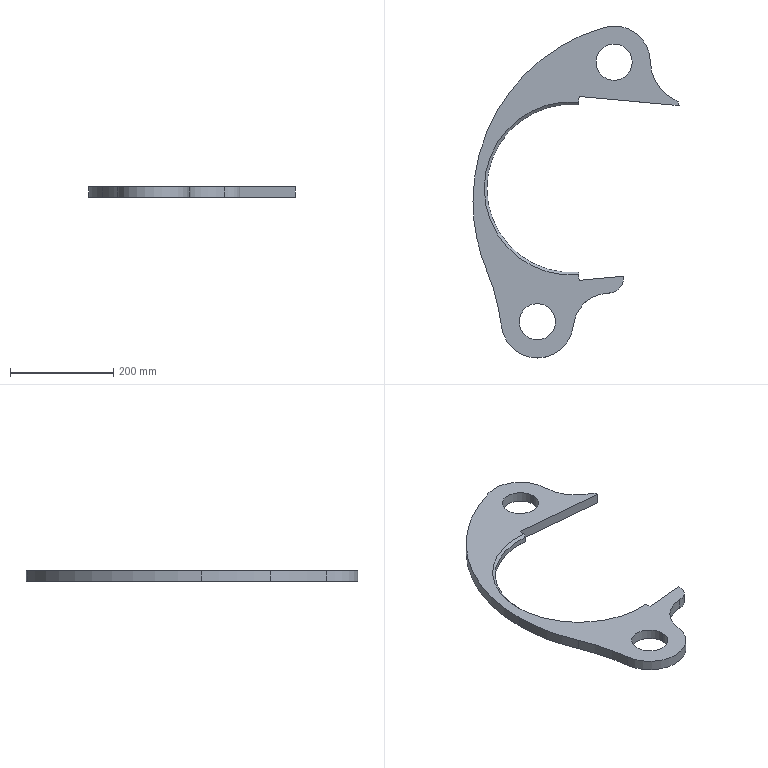Part | SolidWorks | features Chamfer 1, Extrusion 1 | 1 solid | 24 faces | box 398.626 x 642.2 x 20 mm | volume 1286836 mm3 | cylinder 15 | plane 6 | cone 3 | commonest cylinder face diameters 70 x4 140 x3 325 x2 700 x2 20 x1 60 x1
STEP:
#1=CARTESIAN_POINT('',(-162.5,0.,5.));
#2=VERTEX_POINT('',#1);
#3=CARTESIAN_POINT('',(14.745,161.83,5.));
#4=VERTEX_POINT('',#3);
#5=CARTESIAN_POINT('',(0.,0.,5.));
#6=DIRECTION('',(0.,0.,-1.));
#7=DIRECTION('',(1.,0.,0.));
#8=AXIS2_PLACEMENT_3D('',#5,#6,#7);
#9=CIRCLE('',#8,162.5);
#10=EDGE_CURVE('',#2,#4,#9,.T.);
#11=ORIENTED_EDGE('',*,*,#10,.F.);
#12=CARTESIAN_POINT('',(-167.5,0.,0.));
#13=VERTEX_POINT('',#12);
#14=CARTESIAN_POINT('',(-167.5,0.,0.));
#15=DIRECTION('',(-0.7071,0.,-0.7071));
#16=VECTOR('',#15,1000.);
#17=LINE('',#14,#16);
#18=EDGE_CURVE('',#2,#13,#17,.T.);
#19=ORIENTED_EDGE('',*,*,#18,.T.);
#20=CARTESIAN_POINT('',(15.199,166.809,0.));
#21=VERTEX_POINT('',#20);
#22=CARTESIAN_POINT('',(0.,0.,0.));
#23=DIRECTION('',(0.,0.,1.));
#24=DIRECTION('',(1.,0.,0.));
#25=AXIS2_PLACEMENT_3D('',#22,#23,#24);
#26=CIRCLE('',#25,167.5);
#27=EDGE_CURVE('',#21,#13,#26,.T.);
#28=ORIENTED_EDGE('',*,*,#27,.F.);
#29=CARTESIAN_POINT('',(0.,0.,167.5));
#30=DIRECTION('',(0.06416,0.7042,-0.7071));
#31=VECTOR('',#30,1000.);
#32=LINE('',#29,#31);
#33=EDGE_CURVE('',#4,#21,#32,.T.);
#34=ORIENTED_EDGE('',*,*,#33,.F.);
#35=EDGE_LOOP('',(#11,#19,#28,#34));
#36=FACE_OUTER_BOUND('',#35,.T.);
#37=CARTESIAN_POINT('',(0.,0.,0.));
#38=DIRECTION('',(0.,0.,-1.));
#39=DIRECTION('',(-1.,0.,0.));
#40=AXIS2_PLACEMENT_3D('',#37,#38,#39);
#41=CONICAL_SURFACE('',#40,167.5,0.7854);
#42=ADVANCED_FACE('',(#36),#41,.F.);
#43=CARTESIAN_POINT('',(48.7,244.2,20.));
#44=VERTEX_POINT('',#43);
#45=CARTESIAN_POINT('',(118.7,244.2,20.));
#46=VERTEX_POINT('',#45);
#47=CARTESIAN_POINT('',(83.7,244.2,20.));
#48=DIRECTION('',(0.,0.,1.));
#49=DIRECTION('',(1.,0.,0.));
#50=AXIS2_PLACEMENT_3D('',#47,#48,#49);
#51=CIRCLE('',#50,35.);
#52=EDGE_CURVE('',#44,#46,#51,.T.);
#53=ORIENTED_EDGE('',*,*,#52,.T.);
#54=CARTESIAN_POINT('',(118.7,244.2,0.));
#55=VERTEX_POINT('',#54);
#56=CARTESIAN_POINT('',(118.7,244.2,20.));
#57=DIRECTION('',(0.,0.,-1.));
#58=VECTOR('',#57,1000.);
#59=LINE('',#56,#58);
#60=EDGE_CURVE('',#46,#55,#59,.T.);
#61=ORIENTED_EDGE('',*,*,#60,.T.);
#62=CARTESIAN_POINT('',(48.7,244.2,0.));
#63=VERTEX_POINT('',#62);
#64=CARTESIAN_POINT('',(83.7,244.2,0.));
#65=DIRECTION('',(0.,0.,1.));
#66=DIRECTION('',(1.,0.,0.));
#67=AXIS2_PLACEMENT_3D('',#64,#65,#66);
#68=CIRCLE('',#67,35.);
#69=EDGE_CURVE('',#63,#55,#68,.T.);
#70=ORIENTED_EDGE('',*,*,#69,.F.);
#71=CARTESIAN_POINT('',(48.7,244.2,20.));
#72=DIRECTION('',(0.,0.,-1.));
#73=VECTOR('',#72,1000.);
#74=LINE('',#71,#73);
#75=EDGE_CURVE('',#44,#63,#74,.T.);
#76=ORIENTED_EDGE('',*,*,#75,.F.);
#77=EDGE_LOOP('',(#53,#61,#70,#76));
#78=FACE_OUTER_BOUND('',#77,.T.);
#79=CARTESIAN_POINT('',(83.7,244.2,20.));
#80=DIRECTION('',(0.,0.,-1.));
#81=DIRECTION('',(-1.,0.,0.));
#82=AXIS2_PLACEMENT_3D('',#79,#80,#81);
#83=CYLINDRICAL_SURFACE('',#82,35.);
#84=ADVANCED_FACE('',(#78),#83,.F.);
#85=CARTESIAN_POINT('',(-99.8,-258.,20.));
#86=VERTEX_POINT('',#85);
#87=CARTESIAN_POINT('',(-29.8,-258.,20.));
#88=VERTEX_POINT('',#87);
#89=CARTESIAN_POINT('',(-64.8,-258.,20.));
#90=DIRECTION('',(0.,0.,1.));
#91=DIRECTION('',(1.,0.,0.));
#92=AXIS2_PLACEMENT_3D('',#89,#90,#91);
#93=CIRCLE('',#92,35.);
#94=EDGE_CURVE('',#86,#88,#93,.T.);
#95=ORIENTED_EDGE('',*,*,#94,.T.);
#96=CARTESIAN_POINT('',(-29.8,-258.,0.));
#97=VERTEX_POINT('',#96);
#98=CARTESIAN_POINT('',(-29.8,-258.,20.));
#99=DIRECTION('',(0.,0.,-1.));
#100=VECTOR('',#99,1000.);
#101=LINE('',#98,#100);
#102=EDGE_CURVE('',#88,#97,#101,.T.);
#103=ORIENTED_EDGE('',*,*,#102,.T.);
#104=CARTESIAN_POINT('',(-99.8,-258.,0.));
#105=VERTEX_POINT('',#104);
#106=CARTESIAN_POINT('',(-64.8,-258.,0.));
#107=DIRECTION('',(0.,0.,1.));
#108=DIRECTION('',(1.,0.,0.));
#109=AXIS2_PLACEMENT_3D('',#106,#107,#108);
#110=CIRCLE('',#109,35.);
#111=EDGE_CURVE('',#105,#97,#110,.T.);
#112=ORIENTED_EDGE('',*,*,#111,.F.);
#113=CARTESIAN_POINT('',(-99.8,-258.,20.));
#114=DIRECTION('',(0.,0.,-1.));
#115=VECTOR('',#114,1000.);
#116=LINE('',#113,#115);
#117=EDGE_CURVE('',#86,#105,#116,.T.);
#118=ORIENTED_EDGE('',*,*,#117,.F.);
#119=EDGE_LOOP('',(#95,#103,#112,#118));
#120=FACE_OUTER_BOUND('',#119,.T.);
#121=CARTESIAN_POINT('',(-64.8,-258.,20.));
#122=DIRECTION('',(0.,0.,-1.));
#123=DIRECTION('',(-1.,0.,0.));
#124=AXIS2_PLACEMENT_3D('',#121,#122,#123);
#125=CYLINDRICAL_SURFACE('',#124,35.);
#126=ADVANCED_FACE('',(#120),#125,.F.);
#127=CARTESIAN_POINT('',(-189.285,-25.,20.));
#128=VERTEX_POINT('',#127);
#129=CARTESIAN_POINT('',(-162.312,-159.735,20.));
#130=VERTEX_POINT('',#129);
#131=CARTESIAN_POINT('',(160.715,-25.,20.));
#132=DIRECTION('',(0.,0.,1.));
#133=DIRECTION('',(1.,0.,0.));
#134=AXIS2_PLACEMENT_3D('',#131,#132,#133);
#135=CIRCLE('',#134,350.);
#136=EDGE_CURVE('',#128,#130,#135,.T.);
#137=ORIENTED_EDGE('',*,*,#136,.F.);
#138=CARTESIAN_POINT('',(-189.285,-25.,0.));
#139=VERTEX_POINT('',#138);
#140=CARTESIAN_POINT('',(-189.285,-25.,20.));
#141=DIRECTION('',(0.,0.,-1.));
#142=VECTOR('',#141,1000.);
#143=LINE('',#140,#142);
#144=EDGE_CURVE('',#128,#139,#143,.T.);
#145=ORIENTED_EDGE('',*,*,#144,.T.);
#146=CARTESIAN_POINT('',(-162.312,-159.735,0.));
#147=VERTEX_POINT('',#146);
#148=CARTESIAN_POINT('',(160.715,-25.,0.));
#149=DIRECTION('',(0.,0.,1.));
#150=DIRECTION('',(1.,0.,0.));
#151=AXIS2_PLACEMENT_3D('',#148,#149,#150);
#152=CIRCLE('',#151,350.);
#153=EDGE_CURVE('',#139,#147,#152,.T.);
#154=ORIENTED_EDGE('',*,*,#153,.T.);
#155=CARTESIAN_POINT('',(-162.312,-159.735,20.));
#156=DIRECTION('',(0.,0.,-1.));
#157=VECTOR('',#156,1000.);
#158=LINE('',#155,#157);
#159=EDGE_CURVE('',#130,#147,#158,.T.);
#160=ORIENTED_EDGE('',*,*,#159,.F.);
#161=EDGE_LOOP('',(#137,#145,#154,#160));
#162=FACE_OUTER_BOUND('',#161,.T.);
#163=CARTESIAN_POINT('',(160.715,-25.,20.));
#164=DIRECTION('',(0.,0.,-1.));
#165=DIRECTION('',(-1.,0.,0.));
#166=AXIS2_PLACEMENT_3D('',#163,#164,#165);
#167=CYLINDRICAL_SURFACE('',#166,350.);
#168=ADVANCED_FACE('',(#162),#167,.T.);
#169=CARTESIAN_POINT('',(14.745,161.83,15.));
#170=VERTEX_POINT('',#169);
#171=CARTESIAN_POINT('',(-162.5,0.,15.));
#172=VERTEX_POINT('',#171);
#173=CARTESIAN_POINT('',(0.,0.,15.));
#174=DIRECTION('',(0.,0.,1.));
#175=DIRECTION('',(1.,0.,0.));
#176=AXIS2_PLACEMENT_3D('',#173,#174,#175);
#177=CIRCLE('',#176,162.5);
#178=EDGE_CURVE('',#170,#172,#177,.T.);
#179=ORIENTED_EDGE('',*,*,#178,.T.);
#180=CARTESIAN_POINT('',(-162.5,0.,20.));
#181=DIRECTION('',(0.,0.,-1.));
#182=VECTOR('',#181,1000.);
#183=LINE('',#180,#182);
#184=EDGE_CURVE('',#172,#2,#183,.T.);
#185=ORIENTED_EDGE('',*,*,#184,.T.);
#186=ORIENTED_EDGE('',*,*,#10,.T.);
#187=CARTESIAN_POINT('',(14.745,161.83,20.));
#188=DIRECTION('',(0.,0.,-1.));
#189=VECTOR('',#188,1000.);
#190=LINE('',#187,#189);
#191=EDGE_CURVE('',#170,#4,#190,.T.);
#192=ORIENTED_EDGE('',*,*,#191,.F.);
#193=EDGE_LOOP('',(#179,#185,#186,#192));
#194=FACE_OUTER_BOUND('',#193,.T.);
#195=CARTESIAN_POINT('',(0.,0.,20.));
#196=DIRECTION('',(0.,0.,-1.));
#197=DIRECTION('',(-1.,0.,0.));
#198=AXIS2_PLACEMENT_3D('',#195,#196,#197);
#199=CYLINDRICAL_SURFACE('',#198,162.5);
#200=ADVANCED_FACE('',(#194),#199,.F.);
#201=CARTESIAN_POINT('',(72.887,-202.606,0.));
#202=VERTEX_POINT('',#201);
#203=CARTESIAN_POINT('',(4.819,-265.294,0.));
#204=VERTEX_POINT('',#203);
#205=CARTESIAN_POINT('',(74.438,-272.588,0.));
#206=DIRECTION('',(0.,0.,1.));
#207=DIRECTION('',(1.,0.,0.));
#208=AXIS2_PLACEMENT_3D('',#205,#206,#207);
#209=CIRCLE('',#208,70.);
#210=EDGE_CURVE('',#202,#204,#209,.T.);
#211=ORIENTED_EDGE('',*,*,#210,.F.);
#212=CARTESIAN_POINT('',(72.887,-202.606,20.));
#213=VERTEX_POINT('',#212);
#214=CARTESIAN_POINT('',(72.887,-202.606,20.));
#215=DIRECTION('',(0.,0.,-1.));
#216=VECTOR('',#215,1000.);
#217=LINE('',#214,#216);
#218=EDGE_CURVE('',#213,#202,#217,.T.);
#219=ORIENTED_EDGE('',*,*,#218,.F.);
#220=CARTESIAN_POINT('',(4.819,-265.294,20.));
#221=VERTEX_POINT('',#220);
#222=CARTESIAN_POINT('',(74.438,-272.588,20.));
#223=DIRECTION('',(0.,0.,1.));
#224=DIRECTION('',(1.,0.,0.));
#225=AXIS2_PLACEMENT_3D('',#222,#223,#224);
#226=CIRCLE('',#225,70.);
#227=EDGE_CURVE('',#213,#221,#226,.T.);
#228=ORIENTED_EDGE('',*,*,#227,.T.);
#229=CARTESIAN_POINT('',(4.819,-265.294,20.));
#230=DIRECTION('',(0.,0.,-1.));
#231=VECTOR('',#230,1000.);
#232=LINE('',#229,#231);
#233=EDGE_CURVE('',#221,#204,#232,.T.);
#234=ORIENTED_EDGE('',*,*,#233,.T.);
#235=EDGE_LOOP('',(#211,#219,#228,#234));
#236=FACE_OUTER_BOUND('',#235,.T.);
#237=CARTESIAN_POINT('',(74.438,-272.588,20.));
#238=DIRECTION('',(0.,0.,-1.));
#239=DIRECTION('',(-1.,0.,0.));
#240=AXIS2_PLACEMENT_3D('',#237,#238,#239);
#241=CYLINDRICAL_SURFACE('',#240,70.);
#242=ADVANCED_FACE('',(#236),#241,.F.);
#243=CARTESIAN_POINT('',(102.1,-169.9,0.));
#244=VERTEX_POINT('',#243);
#245=CARTESIAN_POINT('',(72.223,-172.613,0.));
#246=DIRECTION('',(0.,0.,1.));
#247=DIRECTION('',(1.,0.,0.));
#248=AXIS2_PLACEMENT_3D('',#245,#246,#247);
#249=CIRCLE('',#248,30.);
#250=EDGE_CURVE('',#202,#244,#249,.T.);
#251=ORIENTED_EDGE('',*,*,#250,.T.);
#252=CARTESIAN_POINT('',(102.1,-169.9,20.));
#253=VERTEX_POINT('',#252);
#254=CARTESIAN_POINT('',(102.1,-169.9,20.));
#255=DIRECTION('',(0.,0.,-1.));
#256=VECTOR('',#255,1000.);
#257=LINE('',#254,#256);
#258=EDGE_CURVE('',#253,#244,#257,.T.);
#259=ORIENTED_EDGE('',*,*,#258,.F.);
#260=CARTESIAN_POINT('',(72.223,-172.613,20.));
#261=DIRECTION('',(0.,0.,1.));
#262=DIRECTION('',(1.,0.,0.));
#263=AXIS2_PLACEMENT_3D('',#260,#261,#262);
#264=CIRCLE('',#263,30.);
#265=EDGE_CURVE('',#213,#253,#264,.T.);
#266=ORIENTED_EDGE('',*,*,#265,.F.);
#267=ORIENTED_EDGE('',*,*,#218,.T.);
#268=EDGE_LOOP('',(#251,#259,#266,#267));
#269=FACE_OUTER_BOUND('',#268,.T.);
#270=CARTESIAN_POINT('',(72.223,-172.613,20.));
#271=DIRECTION('',(0.,0.,-1.));
#272=DIRECTION('',(-1.,0.,0.));
#273=AXIS2_PLACEMENT_3D('',#270,#271,#272);
#274=CYLINDRICAL_SURFACE('',#273,30.);
#275=ADVANCED_FACE('',(#269),#274,.T.);
#276=CARTESIAN_POINT('',(16.2,-177.7,0.));
#277=VERTEX_POINT('',#276);
#278=CARTESIAN_POINT('',(-28.351,-181.745,0.));
#279=DIRECTION('',(0.9959,0.09043,0.));
#280=VECTOR('',#279,1000.);
#281=LINE('',#278,#280);
#282=EDGE_CURVE('',#277,#244,#281,.T.);
#283=ORIENTED_EDGE('',*,*,#282,.F.);
#284=CARTESIAN_POINT('',(16.2,-177.7,20.));
#285=VERTEX_POINT('',#284);
#286=CARTESIAN_POINT('',(16.2,-177.7,20.));
#287=DIRECTION('',(0.,0.,-1.));
#288=VECTOR('',#287,1000.);
#289=LINE('',#286,#288);
#290=EDGE_CURVE('',#285,#277,#289,.T.);
#291=ORIENTED_EDGE('',*,*,#290,.F.);
#292=CARTESIAN_POINT('',(-28.351,-181.745,20.));
#293=DIRECTION('',(0.9959,0.09043,0.));
#294=VECTOR('',#293,1000.);
#295=LINE('',#292,#294);
#296=EDGE_CURVE('',#285,#253,#295,.T.);
#297=ORIENTED_EDGE('',*,*,#296,.T.);
#298=ORIENTED_EDGE('',*,*,#258,.T.);
#299=EDGE_LOOP('',(#283,#291,#297,#298));
#300=FACE_OUTER_BOUND('',#299,.T.);
#301=CARTESIAN_POINT('',(-28.351,-181.745,20.));
#302=DIRECTION('',(-0.09043,0.9959,0.));
#303=DIRECTION('',(-0.9959,-0.09043,0.));
#304=AXIS2_PLACEMENT_3D('',#301,#302,#303);
#305=PLANE('',#304);
#306=ADVANCED_FACE('',(#300),#305,.T.);
#307=CARTESIAN_POINT('',(15.207,-166.808,0.));
#308=VERTEX_POINT('',#307);
#309=CARTESIAN_POINT('',(54.115,-593.599,0.));
#310=DIRECTION('',(-0.09079,0.9959,0.));
#311=VECTOR('',#310,1000.);
#312=LINE('',#309,#311);
#313=EDGE_CURVE('',#277,#308,#312,.T.);
#314=ORIENTED_EDGE('',*,*,#313,.T.);
#315=CARTESIAN_POINT('',(14.753,-161.829,5.));
#316=VERTEX_POINT('',#315);
#317=CARTESIAN_POINT('',(0.,0.,167.5));
#318=DIRECTION('',(-0.0642,0.7042,0.7071));
#319=VECTOR('',#318,1000.);
#320=LINE('',#317,#319);
#321=EDGE_CURVE('',#308,#316,#320,.T.);
#322=ORIENTED_EDGE('',*,*,#321,.T.);
#323=CARTESIAN_POINT('',(14.753,-161.829,15.));
#324=VERTEX_POINT('',#323);
#325=CARTESIAN_POINT('',(14.753,-161.829,20.));
#326=DIRECTION('',(0.,0.,-1.));
#327=VECTOR('',#326,1000.);
#328=LINE('',#325,#327);
#329=EDGE_CURVE('',#324,#316,#328,.T.);
#330=ORIENTED_EDGE('',*,*,#329,.F.);
#331=CARTESIAN_POINT('',(15.207,-166.808,20.));
#332=VERTEX_POINT('',#331);
#333=CARTESIAN_POINT('',(0.,0.,-147.5));
#334=DIRECTION('',(0.0642,-0.7042,0.7071));
#335=VECTOR('',#334,1000.);
#336=LINE('',#333,#335);
#337=EDGE_CURVE('',#324,#332,#336,.T.);
#338=ORIENTED_EDGE('',*,*,#337,.T.);
#339=CARTESIAN_POINT('',(54.115,-593.599,20.));
#340=DIRECTION('',(-0.09079,0.9959,0.));
#341=VECTOR('',#340,1000.);
#342=LINE('',#339,#341);
#343=EDGE_CURVE('',#285,#332,#342,.T.);
#344=ORIENTED_EDGE('',*,*,#343,.F.);
#345=ORIENTED_EDGE('',*,*,#290,.T.);
#346=EDGE_LOOP('',(#314,#322,#330,#338,#344,#345));
#347=FACE_OUTER_BOUND('',#346,.T.);
#348=CARTESIAN_POINT('',(54.115,-593.599,20.));
#349=DIRECTION('',(-0.9959,-0.09079,0.));
#350=DIRECTION('',(0.09079,-0.9959,0.));
#351=AXIS2_PLACEMENT_3D('',#348,#349,#350);
#352=PLANE('',#351);
#353=ADVANCED_FACE('',(#347),#352,.F.);
#354=ORIENTED_EDGE('',*,*,#184,.F.);
#355=CARTESIAN_POINT('',(0.,0.,15.));
#356=DIRECTION('',(0.,0.,1.));
#357=DIRECTION('',(1.,0.,0.));
#358=AXIS2_PLACEMENT_3D('',#355,#356,#357);
#359=CIRCLE('',#358,162.5);
#360=EDGE_CURVE('',#172,#324,#359,.T.);
#361=ORIENTED_EDGE('',*,*,#360,.T.);
#362=ORIENTED_EDGE('',*,*,#329,.T.);
#363=CARTESIAN_POINT('',(0.,0.,5.));
#364=DIRECTION('',(0.,0.,-1.));
#365=DIRECTION('',(1.,0.,0.));
#366=AXIS2_PLACEMENT_3D('',#363,#364,#365);
#367=CIRCLE('',#366,162.5);
#368=EDGE_CURVE('',#316,#2,#367,.T.);
#369=ORIENTED_EDGE('',*,*,#368,.T.);
#370=EDGE_LOOP('',(#354,#361,#362,#369));
#371=FACE_OUTER_BOUND('',#370,.T.);
#372=CARTESIAN_POINT('',(0.,0.,20.));
#373=DIRECTION('',(0.,0.,-1.));
#374=DIRECTION('',(-1.,0.,0.));
#375=AXIS2_PLACEMENT_3D('',#372,#373,#374);
#376=CYLINDRICAL_SURFACE('',#375,162.5);
#377=ADVANCED_FACE('',(#371),#376,.F.);
#378=ORIENTED_EDGE('',*,*,#191,.T.);
#379=ORIENTED_EDGE('',*,*,#33,.T.);
#380=CARTESIAN_POINT('',(16.2,177.8,0.));
#381=VERTEX_POINT('',#380);
#382=CARTESIAN_POINT('',(-53.93,-591.903,0.));
#383=DIRECTION('',(-0.09074,-0.9959,0.));
#384=VECTOR('',#383,1000.);
#385=LINE('',#382,#384);
#386=EDGE_CURVE('',#381,#21,#385,.T.);
#387=ORIENTED_EDGE('',*,*,#386,.F.);
#388=CARTESIAN_POINT('',(16.2,177.8,20.));
#389=VERTEX_POINT('',#388);
#390=CARTESIAN_POINT('',(16.2,177.8,20.));
#391=DIRECTION('',(0.,0.,-1.));
#392=VECTOR('',#391,1000.);
#393=LINE('',#390,#392);
#394=EDGE_CURVE('',#389,#381,#393,.T.);
#395=ORIENTED_EDGE('',*,*,#394,.F.);
#396=CARTESIAN_POINT('',(15.199,166.809,20.));
#397=VERTEX_POINT('',#396);
#398=CARTESIAN_POINT('',(-53.93,-591.903,20.));
#399=DIRECTION('',(-0.09074,-0.9959,0.));
#400=VECTOR('',#399,1000.);
#401=LINE('',#398,#400);
#402=EDGE_CURVE('',#389,#397,#401,.T.);
#403=ORIENTED_EDGE('',*,*,#402,.T.);
#404=CARTESIAN_POINT('',(0.,0.,-147.5));
#405=DIRECTION('',(-0.06416,-0.7042,-0.7071));
#406=VECTOR('',#405,1000.);
#407=LINE('',#404,#406);
#408=EDGE_CURVE('',#397,#170,#407,.T.);
#409=ORIENTED_EDGE('',*,*,#408,.T.);
#410=EDGE_LOOP('',(#378,#379,#387,#395,#403,#409));
#411=FACE_OUTER_BOUND('',#410,.T.);
#412=CARTESIAN_POINT('',(-53.93,-591.903,20.));
#413=DIRECTION('',(0.9959,-0.09074,0.));
#414=DIRECTION('',(0.09074,0.9959,0.));
#415=AXIS2_PLACEMENT_3D('',#412,#413,#414);
#416=PLANE('',#415);
#417=ADVANCED_FACE('',(#411),#416,.T.);
#418=CARTESIAN_POINT('',(209.3,160.2,0.));
#419=VERTEX_POINT('',#418);
#420=CARTESIAN_POINT('',(79.571,172.024,0.));
#421=DIRECTION('',(0.9959,-0.09077,0.));
#422=VECTOR('',#421,1000.);
#423=LINE('',#420,#422);
#424=EDGE_CURVE('',#381,#419,#423,.T.);
#425=ORIENTED_EDGE('',*,*,#424,.T.);
#426=CARTESIAN_POINT('',(209.3,160.2,20.));
#427=VERTEX_POINT('',#426);
#428=CARTESIAN_POINT('',(209.3,160.2,20.));
#429=DIRECTION('',(0.,0.,-1.));
#430=VECTOR('',#429,1000.);
#431=LINE('',#428,#430);
#432=EDGE_CURVE('',#427,#419,#431,.T.);
#433=ORIENTED_EDGE('',*,*,#432,.F.);
#434=CARTESIAN_POINT('',(79.571,172.024,20.));
#435=DIRECTION('',(0.9959,-0.09077,0.));
#436=VECTOR('',#435,1000.);
#437=LINE('',#434,#436);
#438=EDGE_CURVE('',#389,#427,#437,.T.);
#439=ORIENTED_EDGE('',*,*,#438,.F.);
#440=ORIENTED_EDGE('',*,*,#394,.T.);
#441=EDGE_LOOP('',(#425,#433,#439,#440));
#442=FACE_OUTER_BOUND('',#441,.T.);
#443=CARTESIAN_POINT('',(79.571,172.024,20.));
#444=DIRECTION('',(0.09077,0.9959,0.));
#445=DIRECTION('',(-0.9959,0.09077,0.));
#446=AXIS2_PLACEMENT_3D('',#443,#444,#445);
#447=PLANE('',#446);
#448=ADVANCED_FACE('',(#442),#447,.F.);
#449=CARTESIAN_POINT('',(203.48,170.211,0.));
#450=VERTEX_POINT('',#449);
#451=CARTESIAN_POINT('',(199.341,161.108,0.));
#452=DIRECTION('',(0.,0.,1.));
#453=DIRECTION('',(1.,0.,0.));
#454=AXIS2_PLACEMENT_3D('',#451,#452,#453);
#455=CIRCLE('',#454,10.);
#456=EDGE_CURVE('',#419,#450,#455,.T.);
#457=ORIENTED_EDGE('',*,*,#456,.T.);
#458=CARTESIAN_POINT('',(203.48,170.211,20.));
#459=VERTEX_POINT('',#458);
#460=CARTESIAN_POINT('',(203.48,170.211,20.));
#461=DIRECTION('',(0.,0.,-1.));
#462=VECTOR('',#461,1000.);
#463=LINE('',#460,#462);
#464=EDGE_CURVE('',#459,#450,#463,.T.);
#465=ORIENTED_EDGE('',*,*,#464,.F.);
#466=CARTESIAN_POINT('',(199.341,161.108,20.));
#467=DIRECTION('',(0.,0.,1.));
#468=DIRECTION('',(1.,0.,0.));
#469=AXIS2_PLACEMENT_3D('',#466,#467,#468);
#470=CIRCLE('',#469,10.);
#471=EDGE_CURVE('',#427,#459,#470,.T.);
#472=ORIENTED_EDGE('',*,*,#471,.F.);
#473=ORIENTED_EDGE('',*,*,#432,.T.);
#474=EDGE_LOOP('',(#457,#465,#472,#473));
#475=FACE_OUTER_BOUND('',#474,.T.);
#476=CARTESIAN_POINT('',(199.341,161.108,20.));
#477=DIRECTION('',(0.,0.,-1.));
#478=DIRECTION('',(-1.,0.,0.));
#479=AXIS2_PLACEMENT_3D('',#476,#477,#478);
#480=CYLINDRICAL_SURFACE('',#479,10.);
#481=ADVANCED_FACE('',(#475),#480,.T.);
#482=CARTESIAN_POINT('',(153.683,245.73,0.));
#483=VERTEX_POINT('',#482);
#484=CARTESIAN_POINT('',(238.663,247.588,0.));
#485=DIRECTION('',(0.,0.,1.));
#486=DIRECTION('',(1.,0.,0.));
#487=AXIS2_PLACEMENT_3D('',#484,#485,#486);
#488=CIRCLE('',#487,85.);
#489=EDGE_CURVE('',#483,#450,#488,.T.);
#490=ORIENTED_EDGE('',*,*,#489,.F.);
#491=CARTESIAN_POINT('',(153.683,245.73,20.));
#492=VERTEX_POINT('',#491);
#493=CARTESIAN_POINT('',(153.683,245.73,20.));
#494=DIRECTION('',(0.,0.,-1.));
#495=VECTOR('',#494,1000.);
#496=LINE('',#493,#495);
#497=EDGE_CURVE('',#492,#483,#496,.T.);
#498=ORIENTED_EDGE('',*,*,#497,.F.);
#499=CARTESIAN_POINT('',(238.663,247.588,20.));
#500=DIRECTION('',(0.,0.,1.));
#501=DIRECTION('',(1.,0.,0.));
#502=AXIS2_PLACEMENT_3D('',#499,#500,#501);
#503=CIRCLE('',#502,85.);
#504=EDGE_CURVE('',#492,#459,#503,.T.);
#505=ORIENTED_EDGE('',*,*,#504,.T.);
#506=ORIENTED_EDGE('',*,*,#464,.T.);
#507=EDGE_LOOP('',(#490,#498,#505,#506));
#508=FACE_OUTER_BOUND('',#507,.T.);
#509=CARTESIAN_POINT('',(238.663,247.588,20.));
#510=DIRECTION('',(0.,0.,-1.));
#511=DIRECTION('',(-1.,0.,0.));
#512=AXIS2_PLACEMENT_3D('',#509,#510,#511);
#513=CYLINDRICAL_SURFACE('',#512,85.);
#514=ADVANCED_FACE('',(#508),#513,.F.);
#515=CARTESIAN_POINT('',(64.446,311.5,0.));
#516=VERTEX_POINT('',#515);
#517=CARTESIAN_POINT('',(83.7,244.2,0.));
#518=DIRECTION('',(0.,0.,1.));
#519=DIRECTION('',(1.,0.,0.));
#520=AXIS2_PLACEMENT_3D('',#517,#518,#519);
#521=CIRCLE('',#520,70.);
#522=EDGE_CURVE('',#483,#516,#521,.T.);
#523=ORIENTED_EDGE('',*,*,#522,.T.);
#524=CARTESIAN_POINT('',(64.446,311.5,20.));
#525=VERTEX_POINT('',#524);
#526=CARTESIAN_POINT('',(64.446,311.5,20.));
#527=DIRECTION('',(0.,0.,-1.));
#528=VECTOR('',#527,1000.);
#529=LINE('',#526,#528);
#530=EDGE_CURVE('',#525,#516,#529,.T.);
#531=ORIENTED_EDGE('',*,*,#530,.F.);
#532=CARTESIAN_POINT('',(83.7,244.2,20.));
#533=DIRECTION('',(0.,0.,1.));
#534=DIRECTION('',(1.,0.,0.));
#535=AXIS2_PLACEMENT_3D('',#532,#533,#534);
#536=CIRCLE('',#535,70.);
#537=EDGE_CURVE('',#492,#525,#536,.T.);
#538=ORIENTED_EDGE('',*,*,#537,.F.);
#539=ORIENTED_EDGE('',*,*,#497,.T.);
#540=EDGE_LOOP('',(#523,#531,#538,#539));
#541=FACE_OUTER_BOUND('',#540,.T.);
#542=CARTESIAN_POINT('',(83.7,244.2,20.));
#543=DIRECTION('',(0.,0.,-1.));
#544=DIRECTION('',(-1.,0.,0.));
#545=AXIS2_PLACEMENT_3D('',#542,#543,#544);
#546=CYLINDRICAL_SURFACE('',#545,70.);
#547=ADVANCED_FACE('',(#541),#546,.T.);
#548=ORIENTED_EDGE('',*,*,#144,.F.);
#549=CARTESIAN_POINT('',(160.715,-25.,20.));
#550=DIRECTION('',(0.,0.,1.));
#551=DIRECTION('',(1.,0.,0.));
#552=AXIS2_PLACEMENT_3D('',#549,#550,#551);
#553=CIRCLE('',#552,350.);
#554=EDGE_CURVE('',#525,#128,#553,.T.);
#555=ORIENTED_EDGE('',*,*,#554,.F.);
#556=ORIENTED_EDGE('',*,*,#530,.T.);
#557=CARTESIAN_POINT('',(160.715,-25.,0.));
#558=DIRECTION('',(0.,0.,1.));
#559=DIRECTION('',(1.,0.,0.));
#560=AXIS2_PLACEMENT_3D('',#557,#558,#559);
#561=CIRCLE('',#560,350.);
#562=EDGE_CURVE('',#516,#139,#561,.T.);
#563=ORIENTED_EDGE('',*,*,#562,.T.);
#564=EDGE_LOOP('',(#548,#555,#556,#563));
#565=FACE_OUTER_BOUND('',#564,.T.);
#566=CARTESIAN_POINT('',(160.715,-25.,20.));
#567=DIRECTION('',(0.,0.,-1.));
#568=DIRECTION('',(-1.,0.,0.));
#569=AXIS2_PLACEMENT_3D('',#566,#567,#568);
#570=CYLINDRICAL_SURFACE('',#569,350.);
#571=ADVANCED_FACE('',(#565),#570,.T.);
#572=CARTESIAN_POINT('',(-134.306,-266.298,0.));
#573=VERTEX_POINT('',#572);
#574=CARTESIAN_POINT('',(-531.486,-313.717,0.));
#575=DIRECTION('',(0.,0.,1.));
#576=DIRECTION('',(1.,0.,0.));
#577=AXIS2_PLACEMENT_3D('',#574,#575,#576);
#578=CIRCLE('',#577,400.);
#579=EDGE_CURVE('',#573,#147,#578,.T.);
#580=ORIENTED_EDGE('',*,*,#579,.F.);
#581=CARTESIAN_POINT('',(-134.306,-266.298,20.));
#582=VERTEX_POINT('',#581);
#583=CARTESIAN_POINT('',(-134.306,-266.298,20.));
#584=DIRECTION('',(0.,0.,-1.));
#585=VECTOR('',#584,1000.);
#586=LINE('',#583,#585);
#587=EDGE_CURVE('',#582,#573,#586,.T.);
#588=ORIENTED_EDGE('',*,*,#587,.F.);
#589=CARTESIAN_POINT('',(-531.486,-313.717,20.));
#590=DIRECTION('',(0.,0.,1.));
#591=DIRECTION('',(1.,0.,0.));
#592=AXIS2_PLACEMENT_3D('',#589,#590,#591);
#593=CIRCLE('',#592,400.);
#594=EDGE_CURVE('',#582,#130,#593,.T.);
#595=ORIENTED_EDGE('',*,*,#594,.T.);
#596=ORIENTED_EDGE('',*,*,#159,.T.);
#597=EDGE_LOOP('',(#580,#588,#595,#596));
#598=FACE_OUTER_BOUND('',#597,.T.);
#599=CARTESIAN_POINT('',(-531.486,-313.717,20.));
#600=DIRECTION('',(0.,0.,-1.));
#601=DIRECTION('',(-1.,0.,0.));
#602=AXIS2_PLACEMENT_3D('',#599,#600,#601);
#603=CYLINDRICAL_SURFACE('',#602,400.);
#604=ADVANCED_FACE('',(#598),#603,.F.);
#605=ORIENTED_EDGE('',*,*,#102,.F.);
#606=CARTESIAN_POINT('',(-64.8,-258.,20.));
#607=DIRECTION('',(0.,0.,1.));
#608=DIRECTION('',(1.,0.,0.));
#609=AXIS2_PLACEMENT_3D('',#606,#607,#608);
#610=CIRCLE('',#609,35.);
#611=EDGE_CURVE('',#88,#86,#610,.T.);
#612=ORIENTED_EDGE('',*,*,#611,.T.);
#613=ORIENTED_EDGE('',*,*,#117,.T.);
#614=CARTESIAN_POINT('',(-64.8,-258.,0.));
#615=DIRECTION('',(0.,0.,1.));
#616=DIRECTION('',(1.,0.,0.));
#617=AXIS2_PLACEMENT_3D('',#614,#615,#616);
#618=CIRCLE('',#617,35.);
#619=EDGE_CURVE('',#97,#105,#618,.T.);
#620=ORIENTED_EDGE('',*,*,#619,.F.);
#621=EDGE_LOOP('',(#605,#612,#613,#620));
#622=FACE_OUTER_BOUND('',#621,.T.);
#623=CARTESIAN_POINT('',(-64.8,-258.,20.));
#624=DIRECTION('',(0.,0.,-1.));
#625=DIRECTION('',(-1.,0.,0.));
#626=AXIS2_PLACEMENT_3D('',#623,#624,#625);
#627=CYLINDRICAL_SURFACE('',#626,35.);
#628=ADVANCED_FACE('',(#622),#627,.F.);
#629=CARTESIAN_POINT('',(-64.8,-258.,0.));
#630=DIRECTION('',(0.,0.,1.));
#631=DIRECTION('',(1.,0.,0.));
#632=AXIS2_PLACEMENT_3D('',#629,#630,#631);
#633=CIRCLE('',#632,70.);
#634=EDGE_CURVE('',#573,#204,#633,.T.);
#635=ORIENTED_EDGE('',*,*,#634,.T.);
#636=ORIENTED_EDGE('',*,*,#233,.F.);
#637=CARTESIAN_POINT('',(-64.8,-258.,20.));
#638=DIRECTION('',(0.,0.,1.));
#639=DIRECTION('',(1.,0.,0.));
#640=AXIS2_PLACEMENT_3D('',#637,#638,#639);
#641=CIRCLE('',#640,70.);
#642=EDGE_CURVE('',#582,#221,#641,.T.);
#643=ORIENTED_EDGE('',*,*,#642,.F.);
#644=ORIENTED_EDGE('',*,*,#587,.T.);
#645=EDGE_LOOP('',(#635,#636,#643,#644));
#646=FACE_OUTER_BOUND('',#645,.T.);
#647=CARTESIAN_POINT('',(-64.8,-258.,20.));
#648=DIRECTION('',(0.,0.,-1.));
#649=DIRECTION('',(-1.,0.,0.));
#650=AXIS2_PLACEMENT_3D('',#647,#648,#649);
#651=CYLINDRICAL_SURFACE('',#650,70.);
#652=ADVANCED_FACE('',(#646),#651,.T.);
#653=ORIENTED_EDGE('',*,*,#60,.F.);
#654=CARTESIAN_POINT('',(83.7,244.2,20.));
#655=DIRECTION('',(0.,0.,1.));
#656=DIRECTION('',(1.,0.,0.));
#657=AXIS2_PLACEMENT_3D('',#654,#655,#656);
#658=CIRCLE('',#657,35.);
#659=EDGE_CURVE('',#46,#44,#658,.T.);
#660=ORIENTED_EDGE('',*,*,#659,.T.);
#661=ORIENTED_EDGE('',*,*,#75,.T.);
#662=CARTESIAN_POINT('',(83.7,244.2,0.));
#663=DIRECTION('',(0.,0.,1.));
#664=DIRECTION('',(1.,0.,0.));
#665=AXIS2_PLACEMENT_3D('',#662,#663,#664);
#666=CIRCLE('',#665,35.);
#667=EDGE_CURVE('',#55,#63,#666,.T.);
#668=ORIENTED_EDGE('',*,*,#667,.F.);
#669=EDGE_LOOP('',(#653,#660,#661,#668));
#670=FACE_OUTER_BOUND('',#669,.T.);
#671=CARTESIAN_POINT('',(83.7,244.2,20.));
#672=DIRECTION('',(0.,0.,-1.));
#673=DIRECTION('',(-1.,0.,0.));
#674=AXIS2_PLACEMENT_3D('',#671,#672,#673);
#675=CYLINDRICAL_SURFACE('',#674,35.);
#676=ADVANCED_FACE('',(#670),#675,.F.);
#677=ORIENTED_EDGE('',*,*,#343,.T.);
#678=CARTESIAN_POINT('',(0.,0.,20.));
#679=DIRECTION('',(0.,0.,-1.));
#680=DIRECTION('',(1.,0.,0.));
#681=AXIS2_PLACEMENT_3D('',#678,#679,#680);
#682=CIRCLE('',#681,167.5);
#683=EDGE_CURVE('',#332,#397,#682,.T.);
#684=ORIENTED_EDGE('',*,*,#683,.T.);
#685=ORIENTED_EDGE('',*,*,#402,.F.);
#686=ORIENTED_EDGE('',*,*,#438,.T.);
#687=ORIENTED_EDGE('',*,*,#471,.T.);
#688=ORIENTED_EDGE('',*,*,#504,.F.);
#689=ORIENTED_EDGE('',*,*,#537,.T.);
#690=ORIENTED_EDGE('',*,*,#554,.T.);
#691=ORIENTED_EDGE('',*,*,#136,.T.);
#692=ORIENTED_EDGE('',*,*,#594,.F.);
#693=ORIENTED_EDGE('',*,*,#642,.T.);
#694=ORIENTED_EDGE('',*,*,#227,.F.);
#695=ORIENTED_EDGE('',*,*,#265,.T.);
#696=ORIENTED_EDGE('',*,*,#296,.F.);
#697=EDGE_LOOP('',(#677,#684,#685,#686,#687,#688,#689,#690,#691,#692,#693,#694,#695,#696));
#698=FACE_OUTER_BOUND('',#697,.T.);
#699=ORIENTED_EDGE('',*,*,#94,.F.);
#700=ORIENTED_EDGE('',*,*,#611,.F.);
#701=EDGE_LOOP('',(#699,#700));
#702=FACE_BOUND('',#701,.T.);
#703=ORIENTED_EDGE('',*,*,#52,.F.);
#704=ORIENTED_EDGE('',*,*,#659,.F.);
#705=EDGE_LOOP('',(#703,#704));
#706=FACE_BOUND('',#705,.T.);
#707=CARTESIAN_POINT('',(9.417,-597.674,20.));
#708=DIRECTION('',(0.,0.,1.));
#709=DIRECTION('',(1.,0.,0.));
#710=AXIS2_PLACEMENT_3D('',#707,#708,#709);
#711=PLANE('',#710);
#712=ADVANCED_FACE('',(#698,#702,#706),#711,.T.);
#713=ORIENTED_EDGE('',*,*,#386,.T.);
#714=ORIENTED_EDGE('',*,*,#27,.T.);
#715=CARTESIAN_POINT('',(0.,0.,0.));
#716=DIRECTION('',(0.,0.,1.));
#717=DIRECTION('',(1.,0.,0.));
#718=AXIS2_PLACEMENT_3D('',#715,#716,#717);
#719=CIRCLE('',#718,167.5);
#720=EDGE_CURVE('',#13,#308,#719,.T.);
#721=ORIENTED_EDGE('',*,*,#720,.T.);
#722=ORIENTED_EDGE('',*,*,#313,.F.);
#723=ORIENTED_EDGE('',*,*,#282,.T.);
#724=ORIENTED_EDGE('',*,*,#250,.F.);
#725=ORIENTED_EDGE('',*,*,#210,.T.);
#726=ORIENTED_EDGE('',*,*,#634,.F.);
#727=ORIENTED_EDGE('',*,*,#579,.T.);
#728=ORIENTED_EDGE('',*,*,#153,.F.);
#729=ORIENTED_EDGE('',*,*,#562,.F.);
#730=ORIENTED_EDGE('',*,*,#522,.F.);
#731=ORIENTED_EDGE('',*,*,#489,.T.);
#732=ORIENTED_EDGE('',*,*,#456,.F.);
#733=ORIENTED_EDGE('',*,*,#424,.F.);
#734=EDGE_LOOP('',(#713,#714,#721,#722,#723,#724,#725,#726,#727,#728,#729,#730,#731,#732,#733));
#735=FACE_OUTER_BOUND('',#734,.T.);
#736=ORIENTED_EDGE('',*,*,#111,.T.);
#737=ORIENTED_EDGE('',*,*,#619,.T.);
#738=EDGE_LOOP('',(#736,#737));
#739=FACE_BOUND('',#738,.T.);
#740=ORIENTED_EDGE('',*,*,#69,.T.);
#741=ORIENTED_EDGE('',*,*,#667,.T.);
#742=EDGE_LOOP('',(#740,#741));
#743=FACE_BOUND('',#742,.T.);
#744=CARTESIAN_POINT('',(9.417,-597.674,0.));
#745=DIRECTION('',(0.,0.,1.));
#746=DIRECTION('',(1.,0.,0.));
#747=AXIS2_PLACEMENT_3D('',#744,#745,#746);
#748=PLANE('',#747);
#749=ADVANCED_FACE('',(#735,#739,#743),#748,.F.);
#750=ORIENTED_EDGE('',*,*,#18,.F.);
#751=ORIENTED_EDGE('',*,*,#368,.F.);
#752=ORIENTED_EDGE('',*,*,#321,.F.);
#753=ORIENTED_EDGE('',*,*,#720,.F.);
#754=EDGE_LOOP('',(#750,#751,#752,#753));
#755=FACE_OUTER_BOUND('',#754,.T.);
#756=CARTESIAN_POINT('',(0.,0.,0.));
#757=DIRECTION('',(0.,0.,-1.));
#758=DIRECTION('',(-1.,0.,0.));
#759=AXIS2_PLACEMENT_3D('',#756,#757,#758);
#760=CONICAL_SURFACE('',#759,167.5,0.7854);
#761=ADVANCED_FACE('',(#755),#760,.F.);
#762=ORIENTED_EDGE('',*,*,#408,.F.);
#763=ORIENTED_EDGE('',*,*,#683,.F.);
#764=ORIENTED_EDGE('',*,*,#337,.F.);
#765=ORIENTED_EDGE('',*,*,#360,.F.);
#766=ORIENTED_EDGE('',*,*,#178,.F.);
#767=EDGE_LOOP('',(#762,#763,#764,#765,#766));
#768=FACE_OUTER_BOUND('',#767,.T.);
#769=CARTESIAN_POINT('',(0.,0.,15.));
#770=DIRECTION('',(0.,0.,1.));
#771=DIRECTION('',(1.,0.,0.));
#772=AXIS2_PLACEMENT_3D('',#769,#770,#771);
#773=CONICAL_SURFACE('',#772,162.5,0.7854);
#774=ADVANCED_FACE('',(#768),#773,.F.);
#775=CLOSED_SHELL('',(#42,#84,#126,#168,#200,#242,#275,#306,#353,#377,#417,#448,#481,#514,#547,#571,#604,#628,#652,#676,#712,#749,#761,#774));
#776=MANIFOLD_SOLID_BREP('',#775);
#777=CARTESIAN_POINT('',(0.,0.,0.));
#778=DIRECTION('',(0.,0.,1.));
#779=DIRECTION('',(1.,0.,0.));
#780=AXIS2_PLACEMENT_3D('',#777,#778,#779);
#781=(LENGTH_UNIT()NAMED_UNIT(*)SI_UNIT(.MILLI.,.METRE.));
#782=UNCERTAINTY_MEASURE_WITH_UNIT(LENGTH_MEASURE(0.00001),#781,'','');
#783=(NAMED_UNIT(*)PLANE_ANGLE_UNIT()SI_UNIT($,.RADIAN.));
#784=(NAMED_UNIT(*)SI_UNIT($,.STERADIAN.)SOLID_ANGLE_UNIT());
#785=(GEOMETRIC_REPRESENTATION_CONTEXT(3)GLOBAL_UNCERTAINTY_ASSIGNED_CONTEXT((#782))GLOBAL_UNIT_ASSIGNED_CONTEXT((#781,#783,#784))REPRESENTATION_CONTEXT('',''));
#786=ADVANCED_BREP_SHAPE_REPRESENTATION('',(#776,#780),#785);